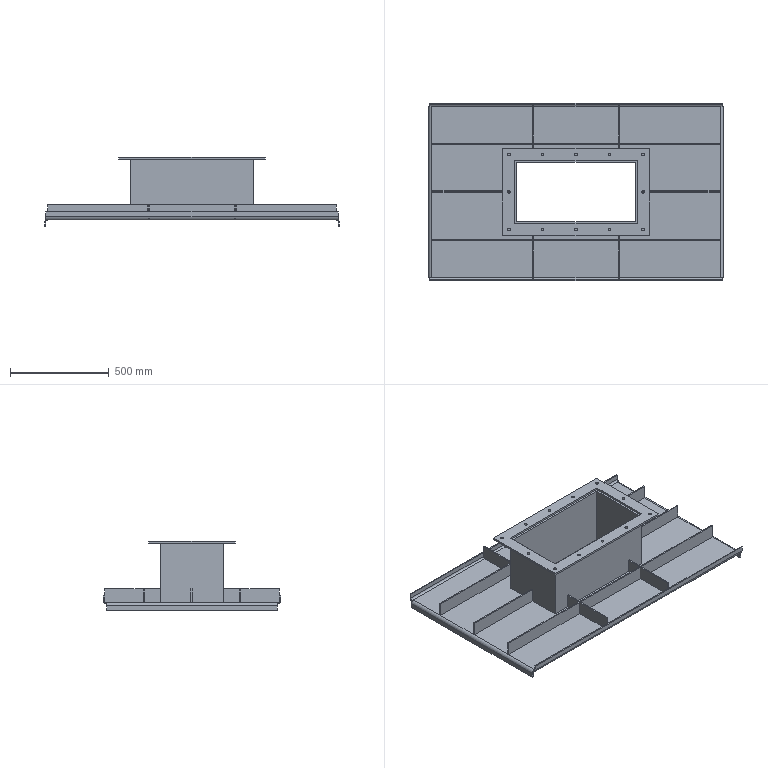Part | SolidWorks | features BossThin 2, EdgeFlange 2, HoleWzd 2, MirrorSolid 2, Cut 1, FlatPattern 1, ICE 1, LPattern 1, MirrorPattern 1, SMBaseFlange 1, SheetMetal 1 | 15 solids | 162 faces | box 1492 x 898 x 350 mm | volume 16578129 mm3 | plane 130 | cylinder 32 | commonest cylinder face diameters 14 x24 20 x4 32 x4